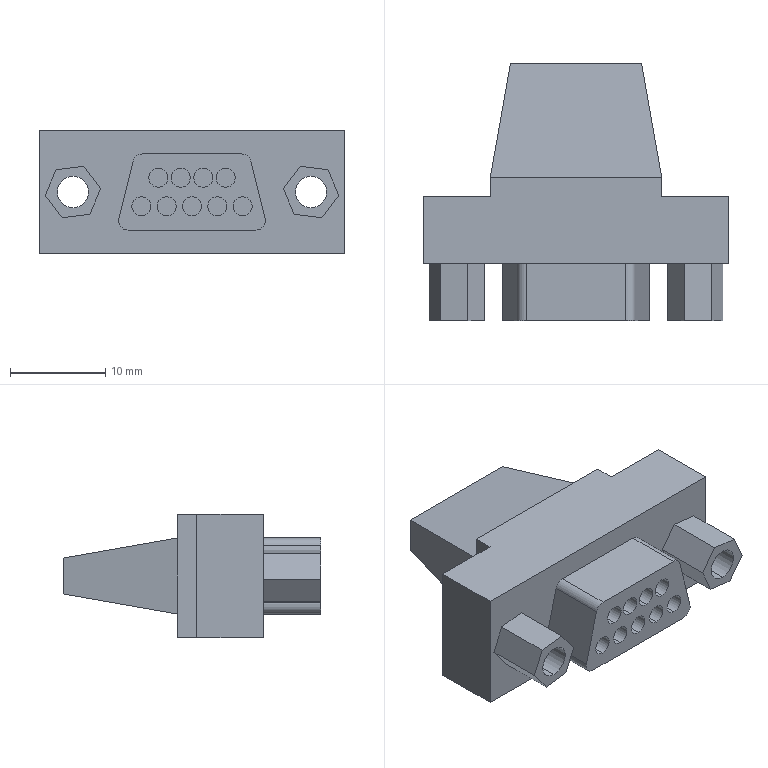Part | STEP file | handheld controller connector DB9-RS232 | 3 solids | 84 faces | box 32 x 27 x 13 mm | volume 4868 mm3 | plane 58 | cylinder 26 | commonest cylinder face diameters 2 x22 3.3 x4